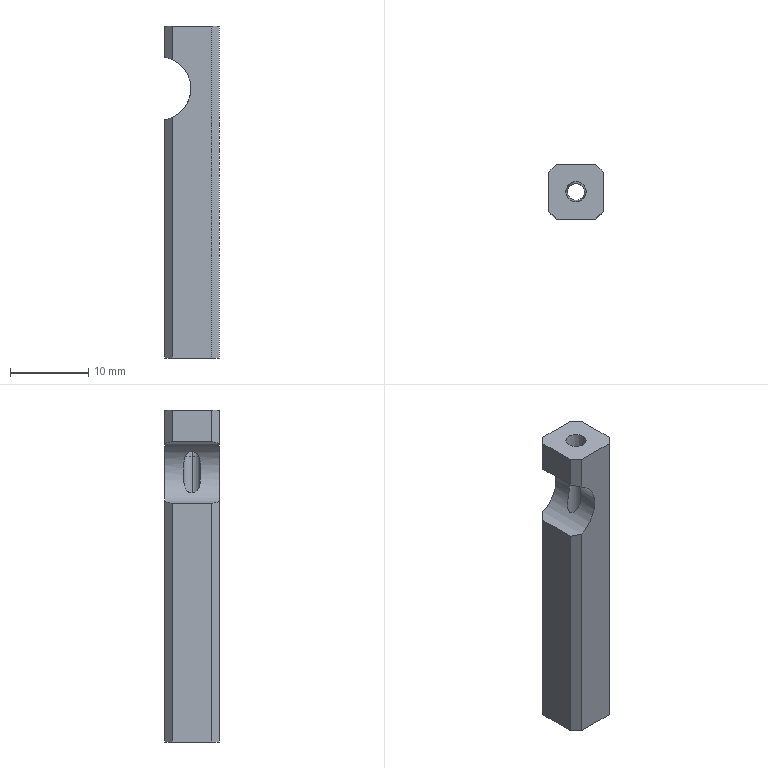Part | SolidWorks | features Chamfer 3, ICE 3, Extrusion 1, MoveFace 1 | 1 solid | 18 faces | box 7 x 7 x 42.5 mm | volume 1702 mm3 | plane 13 | cylinder 3 | cone 2 | commonest cylinder face diameters 2.2 x2 8.159 x1
STEP:
#1=CARTESIAN_POINT('',(-1.122,0.,37.161));
#2=VERTEX_POINT('',#1);
#3=CARTESIAN_POINT('',(-0.6584,-0.8812,36.5));
#4=VERTEX_POINT('',#3);
#5=CARTESIAN_POINT('',(-1.122,0.,37.161));
#6=CARTESIAN_POINT('',(-1.122,-0.1059,37.161));
#7=CARTESIAN_POINT('',(-1.106,-0.2127,37.142));
#8=CARTESIAN_POINT('',(-1.048,-0.4063,37.073));
#9=CARTESIAN_POINT('',(-1.007,-0.4931,37.022));
#10=CARTESIAN_POINT('',(-0.8673,-0.7166,36.838));
#11=CARTESIAN_POINT('',(-0.7581,-0.8141,36.677));
#12=CARTESIAN_POINT('',(-0.6584,-0.8812,36.5));
#13=B_SPLINE_CURVE_WITH_KNOTS('',3,(#5,#6,#7,#8,#9,#10,#11,#12),.UNSPECIFIED.,.F.,.F.,(4,2,2,4),(0.001267,0.001583,0.001898,0.002528),.UNSPECIFIED.);
#14=EDGE_CURVE('',#2,#4,#13,.T.);
#15=ORIENTED_EDGE('',*,*,#14,.F.);
#16=CARTESIAN_POINT('',(-1.3,0.,42.5));
#17=VERTEX_POINT('',#16);
#18=CARTESIAN_POINT('',(-1.1,0.,36.5));
#19=DIRECTION('',(-0.03331,0.,0.9994));
#20=VECTOR('',#19,1000.);
#21=LINE('',#18,#20);
#22=EDGE_CURVE('',#2,#17,#21,.T.);
#23=ORIENTED_EDGE('',*,*,#22,.T.);
#24=CARTESIAN_POINT('',(1.3,0.,42.5));
#25=VERTEX_POINT('',#24);
#26=CARTESIAN_POINT('',(0.,0.,42.5));
#27=DIRECTION('',(0.,0.,-1.));
#28=DIRECTION('',(1.,0.,0.));
#29=AXIS2_PLACEMENT_3D('',#26,#27,#28);
#30=CIRCLE('',#29,1.3);
#31=EDGE_CURVE('',#25,#17,#30,.T.);
#32=ORIENTED_EDGE('',*,*,#31,.F.);
#33=CARTESIAN_POINT('',(1.1,0.,36.5));
#34=VERTEX_POINT('',#33);
#35=CARTESIAN_POINT('',(1.1,0.,36.5));
#36=DIRECTION('',(0.03331,0.,0.9994));
#37=VECTOR('',#36,1000.);
#38=LINE('',#35,#37);
#39=EDGE_CURVE('',#34,#25,#38,.T.);
#40=ORIENTED_EDGE('',*,*,#39,.F.);
#41=CARTESIAN_POINT('',(0.,0.,36.5));
#42=DIRECTION('',(0.,0.,1.));
#43=DIRECTION('',(1.,0.,0.));
#44=AXIS2_PLACEMENT_3D('',#41,#42,#43);
#45=CIRCLE('',#44,1.1);
#46=EDGE_CURVE('',#4,#34,#45,.T.);
#47=ORIENTED_EDGE('',*,*,#46,.F.);
#48=EDGE_LOOP('',(#15,#23,#32,#40,#47));
#49=FACE_OUTER_BOUND('',#48,.T.);
#50=CARTESIAN_POINT('',(0.,0.,36.5));
#51=DIRECTION('',(0.,0.,1.));
#52=DIRECTION('',(1.,0.,0.));
#53=AXIS2_PLACEMENT_3D('',#50,#51,#52);
#54=CONICAL_SURFACE('',#53,1.1,0.03332);
#55=ADVANCED_FACE('',(#49),#54,.F.);
#56=ORIENTED_EDGE('',*,*,#46,.T.);
#57=CARTESIAN_POINT('',(1.1,0.,0.));
#58=VERTEX_POINT('',#57);
#59=CARTESIAN_POINT('',(1.1,0.,40.));
#60=DIRECTION('',(0.,0.,-1.));
#61=VECTOR('',#60,1000.);
#62=LINE('',#59,#61);
#63=EDGE_CURVE('',#34,#58,#62,.T.);
#64=ORIENTED_EDGE('',*,*,#63,.T.);
#65=CARTESIAN_POINT('',(-1.1,0.,0.));
#66=VERTEX_POINT('',#65);
#67=CARTESIAN_POINT('',(0.,0.,0.));
#68=DIRECTION('',(0.,0.,1.));
#69=DIRECTION('',(1.,0.,0.));
#70=AXIS2_PLACEMENT_3D('',#67,#68,#69);
#71=CIRCLE('',#70,1.1);
#72=EDGE_CURVE('',#66,#58,#71,.T.);
#73=ORIENTED_EDGE('',*,*,#72,.F.);
#74=CARTESIAN_POINT('',(-1.1,0.,31.865));
#75=VERTEX_POINT('',#74);
#76=CARTESIAN_POINT('',(-1.1,0.,40.));
#77=DIRECTION('',(0.,0.,-1.));
#78=VECTOR('',#77,1000.);
#79=LINE('',#76,#78);
#80=EDGE_CURVE('',#75,#66,#79,.T.);
#81=ORIENTED_EDGE('',*,*,#80,.F.);
#82=CARTESIAN_POINT('',(-0.6584,-0.8812,36.5));
#83=CARTESIAN_POINT('',(-0.6059,-0.9204,36.407));
#84=CARTESIAN_POINT('',(-0.555,-0.9512,36.307));
#85=CARTESIAN_POINT('',(-0.4617,-0.9998,36.105));
#86=CARTESIAN_POINT('',(-0.419,-1.018,36.001));
#87=CARTESIAN_POINT('',(-0.3034,-1.061,35.683));
#88=CARTESIAN_POINT('',(-0.2428,-1.074,35.461));
#89=CARTESIAN_POINT('',(-0.1607,-1.089,35.014));
#90=CARTESIAN_POINT('',(-0.1385,-1.091,34.789));
#91=CARTESIAN_POINT('',(-0.1316,-1.092,34.336));
#92=CARTESIAN_POINT('',(-0.1473,-1.091,34.106));
#93=CARTESIAN_POINT('',(-0.2161,-1.079,33.657));
#94=CARTESIAN_POINT('',(-0.2688,-1.069,33.438));
#95=CARTESIAN_POINT('',(-0.4097,-1.024,33.01));
#96=CARTESIAN_POINT('',(-0.4996,-0.9875,32.799));
#97=CARTESIAN_POINT('',(-0.6524,-0.8878,32.508));
#98=CARTESIAN_POINT('',(-0.7068,-0.8462,32.414));
#99=CARTESIAN_POINT('',(-0.8149,-0.7426,32.242));
#100=CARTESIAN_POINT('',(-0.869,-0.6808,32.163));
#101=CARTESIAN_POINT('',(-0.9706,-0.5258,32.024));
#102=CARTESIAN_POINT('',(-1.016,-0.435,31.967));
#103=CARTESIAN_POINT('',(-1.065,-0.2806,31.906));
#104=CARTESIAN_POINT('',(-1.078,-0.2271,31.891));
#105=CARTESIAN_POINT('',(-1.095,-0.1158,31.87));
#106=CARTESIAN_POINT('',(-1.1,-0.05736,31.865));
#107=CARTESIAN_POINT('',(-1.1,0.,31.865));
#108=B_SPLINE_CURVE_WITH_KNOTS('',3,(#82,#83,#84,#85,#86,#87,#88,#89,#90,#91,#92,#93,#94,#95,#96,#97,#98,#99,#100,#101,#102,#103,#104,#105,#106,#107),.UNSPECIFIED.,.F.,.F.,(4,2,2,2,2,2,2,2,2,2,2,2,4),(0.001246,0.001589,0.001932,0.002617,0.003303,0.003989,0.004675,0.00536,0.005703,0.006046,0.006389,0.00656,0.006732),.UNSPECIFIED.);
#109=EDGE_CURVE('',#4,#75,#108,.T.);
#110=ORIENTED_EDGE('',*,*,#109,.F.);
#111=EDGE_LOOP('',(#56,#64,#73,#81,#110));
#112=FACE_OUTER_BOUND('',#111,.T.);
#113=CARTESIAN_POINT('',(0.,0.,40.));
#114=DIRECTION('',(0.,0.,-1.));
#115=DIRECTION('',(-1.,0.,0.));
#116=AXIS2_PLACEMENT_3D('',#113,#114,#115);
#117=CYLINDRICAL_SURFACE('',#116,1.1);
#118=ADVANCED_FACE('',(#112),#117,.F.);
#119=CARTESIAN_POINT('',(-3.5,2.5,30.483));
#120=VERTEX_POINT('',#119);
#121=CARTESIAN_POINT('',(-3.5,-2.5,30.483));
#122=VERTEX_POINT('',#121);
#123=CARTESIAN_POINT('',(-3.5,-9.5,30.483));
#124=DIRECTION('',(0.,-1.,0.));
#125=VECTOR('',#124,1000.);
#126=LINE('',#123,#125);
#127=EDGE_CURVE('',#120,#122,#126,.T.);
#128=ORIENTED_EDGE('',*,*,#127,.F.);
#129=CARTESIAN_POINT('',(-3.5,2.5,0.));
#130=VERTEX_POINT('',#129);
#131=CARTESIAN_POINT('',(-3.5,2.5,-9.899));
#132=DIRECTION('',(0.,0.,-1.));
#133=VECTOR('',#132,1000.);
#134=LINE('',#131,#133);
#135=EDGE_CURVE('',#120,#130,#134,.T.);
#136=ORIENTED_EDGE('',*,*,#135,.T.);
#137=CARTESIAN_POINT('',(-3.5,-2.5,0.));
#138=VERTEX_POINT('',#137);
#139=CARTESIAN_POINT('',(-3.5,-3.5,0.));
#140=DIRECTION('',(0.,1.,0.));
#141=VECTOR('',#140,1000.);
#142=LINE('',#139,#141);
#143=EDGE_CURVE('',#138,#130,#142,.T.);
#144=ORIENTED_EDGE('',*,*,#143,.F.);
#145=CARTESIAN_POINT('',(-3.5,-2.5,-9.899));
#146=DIRECTION('',(0.,0.,1.));
#147=VECTOR('',#146,1000.);
#148=LINE('',#145,#147);
#149=EDGE_CURVE('',#138,#122,#148,.T.);
#150=ORIENTED_EDGE('',*,*,#149,.T.);
#151=EDGE_LOOP('',(#128,#136,#144,#150));
#152=FACE_OUTER_BOUND('',#151,.T.);
#153=CARTESIAN_POINT('',(-3.5,-3.5,-9.899));
#154=DIRECTION('',(-1.,0.,0.));
#155=DIRECTION('',(0.,0.,1.));
#156=AXIS2_PLACEMENT_3D('',#153,#154,#155);
#157=PLANE('',#156);
#158=ADVANCED_FACE('',(#152),#157,.T.);
#159=CARTESIAN_POINT('',(-2.5,3.5,30.798));
#160=VERTEX_POINT('',#159);
#161=CARTESIAN_POINT('',(-2.5,3.5,30.798));
#162=CARTESIAN_POINT('',(-2.819,3.181,30.65));
#163=CARTESIAN_POINT('',(-3.154,2.846,30.545));
#164=CARTESIAN_POINT('',(-3.5,2.5,30.483));
#165=(BOUNDED_CURVE()B_SPLINE_CURVE(3,(#161,#162,#163,#164),.UNSPECIFIED.,.F.,.T.)B_SPLINE_CURVE_WITH_KNOTS((4,4),(1.137,1.395),.UNSPECIFIED.)CURVE()GEOMETRIC_REPRESENTATION_ITEM()RATIONAL_B_SPLINE_CURVE((1.,0.9945,0.9945,1.))REPRESENTATION_ITEM(''));
#166=EDGE_CURVE('',#160,#120,#165,.T.);
#167=ORIENTED_EDGE('',*,*,#166,.F.);
#168=CARTESIAN_POINT('',(-2.5,3.5,0.));
#169=VERTEX_POINT('',#168);
#170=CARTESIAN_POINT('',(-2.5,3.5,-9.899));
#171=DIRECTION('',(0.,0.,1.));
#172=VECTOR('',#171,1000.);
#173=LINE('',#170,#172);
#174=EDGE_CURVE('',#169,#160,#173,.T.);
#175=ORIENTED_EDGE('',*,*,#174,.F.);
#176=CARTESIAN_POINT('',(-2.5,3.5,0.));
#177=DIRECTION('',(0.7071,0.7071,0.));
#178=VECTOR('',#177,1000.);
#179=LINE('',#176,#178);
#180=EDGE_CURVE('',#130,#169,#179,.T.);
#181=ORIENTED_EDGE('',*,*,#180,.F.);
#182=ORIENTED_EDGE('',*,*,#135,.F.);
#183=EDGE_LOOP('',(#167,#175,#181,#182));
#184=FACE_OUTER_BOUND('',#183,.T.);
#185=CARTESIAN_POINT('',(-2.5,3.5,-9.899));
#186=DIRECTION('',(0.7071,-0.7071,0.));
#187=DIRECTION('',(0.,0.,1.));
#188=AXIS2_PLACEMENT_3D('',#185,#186,#187);
#189=PLANE('',#188);
#190=ADVANCED_FACE('',(#184),#189,.F.);
#191=CARTESIAN_POINT('',(-2.5,-3.5,30.798));
#192=VERTEX_POINT('',#191);
#193=CARTESIAN_POINT('',(-3.5,-2.5,30.483));
#194=CARTESIAN_POINT('',(-3.154,-2.846,30.545));
#195=CARTESIAN_POINT('',(-2.819,-3.181,30.65));
#196=CARTESIAN_POINT('',(-2.5,-3.5,30.798));
#197=(BOUNDED_CURVE()B_SPLINE_CURVE(3,(#193,#194,#195,#196),.UNSPECIFIED.,.F.,.T.)B_SPLINE_CURVE_WITH_KNOTS((4,4),(1.747,2.004),.UNSPECIFIED.)CURVE()GEOMETRIC_REPRESENTATION_ITEM()RATIONAL_B_SPLINE_CURVE((1.,0.9945,0.9945,1.))REPRESENTATION_ITEM(''));
#198=EDGE_CURVE('',#122,#192,#197,.T.);
#199=ORIENTED_EDGE('',*,*,#198,.F.);
#200=ORIENTED_EDGE('',*,*,#149,.F.);
#201=CARTESIAN_POINT('',(-2.5,-3.5,0.));
#202=VERTEX_POINT('',#201);
#203=CARTESIAN_POINT('',(-3.5,-2.5,0.));
#204=DIRECTION('',(-0.7071,0.7071,0.));
#205=VECTOR('',#204,1000.);
#206=LINE('',#203,#205);
#207=EDGE_CURVE('',#202,#138,#206,.T.);
#208=ORIENTED_EDGE('',*,*,#207,.F.);
#209=CARTESIAN_POINT('',(-2.5,-3.5,-9.899));
#210=DIRECTION('',(0.,0.,-1.));
#211=VECTOR('',#210,1000.);
#212=LINE('',#209,#211);
#213=EDGE_CURVE('',#192,#202,#212,.T.);
#214=ORIENTED_EDGE('',*,*,#213,.F.);
#215=EDGE_LOOP('',(#199,#200,#208,#214));
#216=FACE_OUTER_BOUND('',#215,.T.);
#217=CARTESIAN_POINT('',(-3.5,-2.5,-9.899));
#218=DIRECTION('',(0.7071,0.7071,0.));
#219=DIRECTION('',(0.,0.,1.));
#220=AXIS2_PLACEMENT_3D('',#217,#218,#219);
#221=PLANE('',#220);
#222=ADVANCED_FACE('',(#216),#221,.F.);
#223=ORIENTED_EDGE('',*,*,#31,.T.);
#224=CARTESIAN_POINT('',(0.,0.,42.5));
#225=DIRECTION('',(0.,0.,-1.));
#226=DIRECTION('',(1.,0.,0.));
#227=AXIS2_PLACEMENT_3D('',#224,#225,#226);
#228=CIRCLE('',#227,1.3);
#229=EDGE_CURVE('',#17,#25,#228,.T.);
#230=ORIENTED_EDGE('',*,*,#229,.T.);
#231=EDGE_LOOP('',(#223,#230));
#232=FACE_BOUND('',#231,.T.);
#233=CARTESIAN_POINT('',(3.5,-2.5,42.5));
#234=VERTEX_POINT('',#233);
#235=CARTESIAN_POINT('',(3.5,2.5,42.5));
#236=VERTEX_POINT('',#235);
#237=CARTESIAN_POINT('',(3.5,0.,42.5));
#238=DIRECTION('',(0.,1.,0.));
#239=VECTOR('',#238,1000.);
#240=LINE('',#237,#239);
#241=EDGE_CURVE('',#234,#236,#240,.T.);
#242=ORIENTED_EDGE('',*,*,#241,.T.);
#243=CARTESIAN_POINT('',(2.5,3.5,42.5));
#244=VERTEX_POINT('',#243);
#245=CARTESIAN_POINT('',(3.,3.,42.5));
#246=DIRECTION('',(-0.7071,0.7071,0.));
#247=VECTOR('',#246,1000.);
#248=LINE('',#245,#247);
#249=EDGE_CURVE('',#236,#244,#248,.T.);
#250=ORIENTED_EDGE('',*,*,#249,.T.);
#251=CARTESIAN_POINT('',(-2.5,3.5,42.5));
#252=VERTEX_POINT('',#251);
#253=CARTESIAN_POINT('',(0.,3.5,42.5));
#254=DIRECTION('',(-1.,0.,0.));
#255=VECTOR('',#254,1000.);
#256=LINE('',#253,#255);
#257=EDGE_CURVE('',#244,#252,#256,.T.);
#258=ORIENTED_EDGE('',*,*,#257,.T.);
#259=CARTESIAN_POINT('',(-3.5,2.5,42.5));
#260=VERTEX_POINT('',#259);
#261=CARTESIAN_POINT('',(-3.,3.,42.5));
#262=DIRECTION('',(-0.7071,-0.7071,0.));
#263=VECTOR('',#262,1000.);
#264=LINE('',#261,#263);
#265=EDGE_CURVE('',#252,#260,#264,.T.);
#266=ORIENTED_EDGE('',*,*,#265,.T.);
#267=CARTESIAN_POINT('',(-3.5,-2.5,42.5));
#268=VERTEX_POINT('',#267);
#269=CARTESIAN_POINT('',(-3.5,0.,42.5));
#270=DIRECTION('',(0.,-1.,0.));
#271=VECTOR('',#270,1000.);
#272=LINE('',#269,#271);
#273=EDGE_CURVE('',#260,#268,#272,.T.);
#274=ORIENTED_EDGE('',*,*,#273,.T.);
#275=CARTESIAN_POINT('',(-2.5,-3.5,42.5));
#276=VERTEX_POINT('',#275);
#277=CARTESIAN_POINT('',(-3.,-3.,42.5));
#278=DIRECTION('',(0.7071,-0.7071,0.));
#279=VECTOR('',#278,1000.);
#280=LINE('',#277,#279);
#281=EDGE_CURVE('',#268,#276,#280,.T.);
#282=ORIENTED_EDGE('',*,*,#281,.T.);
#283=CARTESIAN_POINT('',(2.5,-3.5,42.5));
#284=VERTEX_POINT('',#283);
#285=CARTESIAN_POINT('',(0.,-3.5,42.5));
#286=DIRECTION('',(1.,0.,0.));
#287=VECTOR('',#286,1000.);
#288=LINE('',#285,#287);
#289=EDGE_CURVE('',#276,#284,#288,.T.);
#290=ORIENTED_EDGE('',*,*,#289,.T.);
#291=CARTESIAN_POINT('',(3.,-3.,42.5));
#292=DIRECTION('',(0.7071,0.7071,0.));
#293=VECTOR('',#292,1000.);
#294=LINE('',#291,#293);
#295=EDGE_CURVE('',#284,#234,#294,.T.);
#296=ORIENTED_EDGE('',*,*,#295,.T.);
#297=EDGE_LOOP('',(#242,#250,#258,#266,#274,#282,#290,#296));
#298=FACE_OUTER_BOUND('',#297,.T.);
#299=CARTESIAN_POINT('',(0.,0.,42.5));
#300=DIRECTION('',(0.,0.,1.));
#301=DIRECTION('',(1.,0.,0.));
#302=AXIS2_PLACEMENT_3D('',#299,#300,#301);
#303=PLANE('',#302);
#304=ADVANCED_FACE('',(#232,#298),#303,.T.);
#305=CARTESIAN_POINT('',(2.5,3.5,0.));
#306=VERTEX_POINT('',#305);
#307=CARTESIAN_POINT('',(-3.5,3.5,0.));
#308=DIRECTION('',(1.,0.,0.));
#309=VECTOR('',#308,1000.);
#310=LINE('',#307,#309);
#311=EDGE_CURVE('',#169,#306,#310,.T.);
#312=ORIENTED_EDGE('',*,*,#311,.T.);
#313=CARTESIAN_POINT('',(3.5,2.5,0.));
#314=VERTEX_POINT('',#313);
#315=CARTESIAN_POINT('',(3.5,2.5,0.));
#316=DIRECTION('',(0.7071,-0.7071,0.));
#317=VECTOR('',#316,1000.);
#318=LINE('',#315,#317);
#319=EDGE_CURVE('',#306,#314,#318,.T.);
#320=ORIENTED_EDGE('',*,*,#319,.T.);
#321=CARTESIAN_POINT('',(3.5,-2.5,0.));
#322=VERTEX_POINT('',#321);
#323=CARTESIAN_POINT('',(3.5,-3.5,0.));
#324=DIRECTION('',(0.,-1.,0.));
#325=VECTOR('',#324,1000.);
#326=LINE('',#323,#325);
#327=EDGE_CURVE('',#314,#322,#326,.T.);
#328=ORIENTED_EDGE('',*,*,#327,.T.);
#329=CARTESIAN_POINT('',(2.5,-3.5,0.));
#330=VERTEX_POINT('',#329);
#331=CARTESIAN_POINT('',(2.5,-3.5,0.));
#332=DIRECTION('',(-0.7071,-0.7071,0.));
#333=VECTOR('',#332,1000.);
#334=LINE('',#331,#333);
#335=EDGE_CURVE('',#322,#330,#334,.T.);
#336=ORIENTED_EDGE('',*,*,#335,.T.);
#337=CARTESIAN_POINT('',(-3.5,-3.5,0.));
#338=DIRECTION('',(-1.,0.,0.));
#339=VECTOR('',#338,1000.);
#340=LINE('',#337,#339);
#341=EDGE_CURVE('',#330,#202,#340,.T.);
#342=ORIENTED_EDGE('',*,*,#341,.T.);
#343=ORIENTED_EDGE('',*,*,#207,.T.);
#344=ORIENTED_EDGE('',*,*,#143,.T.);
#345=ORIENTED_EDGE('',*,*,#180,.T.);
#346=EDGE_LOOP('',(#312,#320,#328,#336,#342,#343,#344,#345));
#347=FACE_OUTER_BOUND('',#346,.T.);
#348=ORIENTED_EDGE('',*,*,#72,.T.);
#349=CARTESIAN_POINT('',(0.,0.,0.));
#350=DIRECTION('',(0.,0.,1.));
#351=DIRECTION('',(1.,0.,0.));
#352=AXIS2_PLACEMENT_3D('',#349,#350,#351);
#353=CIRCLE('',#352,1.1);
#354=EDGE_CURVE('',#58,#66,#353,.T.);
#355=ORIENTED_EDGE('',*,*,#354,.T.);
#356=EDGE_LOOP('',(#348,#355));
#357=FACE_BOUND('',#356,.T.);
#358=CARTESIAN_POINT('',(0.,0.,0.));
#359=DIRECTION('',(0.,0.,1.));
#360=DIRECTION('',(1.,0.,0.));
#361=AXIS2_PLACEMENT_3D('',#358,#359,#360);
#362=PLANE('',#361);
#363=ADVANCED_FACE('',(#347,#357),#362,.F.);
#364=ORIENTED_EDGE('',*,*,#63,.F.);
#365=CARTESIAN_POINT('',(-0.6584,0.8812,36.5));
#366=VERTEX_POINT('',#365);
#367=CARTESIAN_POINT('',(0.,0.,36.5));
#368=DIRECTION('',(0.,0.,1.));
#369=DIRECTION('',(1.,0.,0.));
#370=AXIS2_PLACEMENT_3D('',#367,#368,#369);
#371=CIRCLE('',#370,1.1);
#372=EDGE_CURVE('',#34,#366,#371,.T.);
#373=ORIENTED_EDGE('',*,*,#372,.T.);
#374=CARTESIAN_POINT('',(-1.1,0.,31.865));
#375=CARTESIAN_POINT('',(-1.1,0.1143,31.865));
#376=CARTESIAN_POINT('',(-1.081,0.2291,31.886));
#377=CARTESIAN_POINT('',(-1.016,0.4346,31.966));
#378=CARTESIAN_POINT('',(-0.9706,0.5258,32.024));
#379=CARTESIAN_POINT('',(-0.8188,0.7573,32.232));
#380=CARTESIAN_POINT('',(-0.703,0.8546,32.411));
#381=CARTESIAN_POINT('',(-0.5007,0.9868,32.797));
#382=CARTESIAN_POINT('',(-0.4107,1.023,33.007));
#383=CARTESIAN_POINT('',(-0.2692,1.069,33.436));
#384=CARTESIAN_POINT('',(-0.2163,1.079,33.656));
#385=CARTESIAN_POINT('',(-0.1472,1.091,34.107));
#386=CARTESIAN_POINT('',(-0.1316,1.092,34.335));
#387=CARTESIAN_POINT('',(-0.1385,1.091,34.788));
#388=CARTESIAN_POINT('',(-0.1607,1.089,35.015));
#389=CARTESIAN_POINT('',(-0.2436,1.074,35.464));
#390=CARTESIAN_POINT('',(-0.3033,1.061,35.683));
#391=CARTESIAN_POINT('',(-0.4574,1.004,36.106));
#392=CARTESIAN_POINT('',(-0.5533,0.9598,36.313));
#393=CARTESIAN_POINT('',(-0.6584,0.8812,36.5));
#394=B_SPLINE_CURVE_WITH_KNOTS('',3,(#374,#375,#376,#377,#378,#379,#380,#381,#382,#383,#384,#385,#386,#387,#388,#389,#390,#391,#392,#393),.UNSPECIFIED.,.F.,.F.,(4,2,2,2,2,2,2,2,2,4),(0.006732,0.007073,0.007415,0.008098,0.008782,0.009465,0.01015,0.01083,0.01152,0.0122),.UNSPECIFIED.);
#395=EDGE_CURVE('',#75,#366,#394,.T.);
#396=ORIENTED_EDGE('',*,*,#395,.F.);
#397=ORIENTED_EDGE('',*,*,#80,.T.);
#398=ORIENTED_EDGE('',*,*,#354,.F.);
#399=EDGE_LOOP('',(#364,#373,#396,#397,#398));
#400=FACE_OUTER_BOUND('',#399,.T.);
#401=CARTESIAN_POINT('',(0.,0.,40.));
#402=DIRECTION('',(0.,0.,-1.));
#403=DIRECTION('',(-1.,0.,0.));
#404=AXIS2_PLACEMENT_3D('',#401,#402,#403);
#405=CYLINDRICAL_SURFACE('',#404,1.1);
#406=ADVANCED_FACE('',(#400),#405,.F.);
#407=CARTESIAN_POINT('',(-2.5,3.5,38.202));
#408=VERTEX_POINT('',#407);
#409=CARTESIAN_POINT('',(-4.214,3.5,34.5));
#410=DIRECTION('',(0.,1.,0.));
#411=DIRECTION('',(0.,0.,1.));
#412=AXIS2_PLACEMENT_3D('',#409,#410,#411);
#413=CIRCLE('',#412,4.08);
#414=EDGE_CURVE('',#408,#160,#413,.T.);
#415=ORIENTED_EDGE('',*,*,#414,.F.);
#416=CARTESIAN_POINT('',(-2.5,3.5,-9.899));
#417=DIRECTION('',(0.,0.,1.));
#418=VECTOR('',#417,1000.);
#419=LINE('',#416,#418);
#420=EDGE_CURVE('',#408,#252,#419,.T.);
#421=ORIENTED_EDGE('',*,*,#420,.T.);
#422=ORIENTED_EDGE('',*,*,#257,.F.);
#423=CARTESIAN_POINT('',(2.5,3.5,-9.899));
#424=DIRECTION('',(0.,0.,-1.));
#425=VECTOR('',#424,1000.);
#426=LINE('',#423,#425);
#427=EDGE_CURVE('',#244,#306,#426,.T.);
#428=ORIENTED_EDGE('',*,*,#427,.T.);
#429=ORIENTED_EDGE('',*,*,#311,.F.);
#430=ORIENTED_EDGE('',*,*,#174,.T.);
#431=EDGE_LOOP('',(#415,#421,#422,#428,#429,#430));
#432=FACE_OUTER_BOUND('',#431,.T.);
#433=CARTESIAN_POINT('',(-3.5,3.5,-9.899));
#434=DIRECTION('',(0.,1.,0.));
#435=DIRECTION('',(0.,0.,1.));
#436=AXIS2_PLACEMENT_3D('',#433,#434,#435);
#437=PLANE('',#436);
#438=ADVANCED_FACE('',(#432),#437,.T.);
#439=CARTESIAN_POINT('',(-3.5,-2.5,38.517));
#440=VERTEX_POINT('',#439);
#441=CARTESIAN_POINT('',(-3.5,2.5,38.517));
#442=VERTEX_POINT('',#441);
#443=CARTESIAN_POINT('',(-3.5,-9.5,38.517));
#444=DIRECTION('',(0.,1.,0.));
#445=VECTOR('',#444,1000.);
#446=LINE('',#443,#445);
#447=EDGE_CURVE('',#440,#442,#446,.T.);
#448=ORIENTED_EDGE('',*,*,#447,.F.);
#449=CARTESIAN_POINT('',(-3.5,-2.5,-9.899));
#450=DIRECTION('',(0.,0.,1.));
#451=VECTOR('',#450,1000.);
#452=LINE('',#449,#451);
#453=EDGE_CURVE('',#440,#268,#452,.T.);
#454=ORIENTED_EDGE('',*,*,#453,.T.);
#455=ORIENTED_EDGE('',*,*,#273,.F.);
#456=CARTESIAN_POINT('',(-3.5,2.5,-9.899));
#457=DIRECTION('',(0.,0.,-1.));
#458=VECTOR('',#457,1000.);
#459=LINE('',#456,#458);
#460=EDGE_CURVE('',#260,#442,#459,.T.);
#461=ORIENTED_EDGE('',*,*,#460,.T.);
#462=EDGE_LOOP('',(#448,#454,#455,#461));
#463=FACE_OUTER_BOUND('',#462,.T.);
#464=CARTESIAN_POINT('',(-3.5,-3.5,-9.899));
#465=DIRECTION('',(-1.,0.,0.));
#466=DIRECTION('',(0.,0.,1.));
#467=AXIS2_PLACEMENT_3D('',#464,#465,#466);
#468=PLANE('',#467);
#469=ADVANCED_FACE('',(#463),#468,.T.);
#470=CARTESIAN_POINT('',(-2.5,-3.5,38.202));
#471=VERTEX_POINT('',#470);
#472=CARTESIAN_POINT('',(-4.214,-3.5,34.5));
#473=DIRECTION('',(0.,-1.,0.));
#474=DIRECTION('',(0.,0.,-1.));
#475=AXIS2_PLACEMENT_3D('',#472,#473,#474);
#476=CIRCLE('',#475,4.08);
#477=EDGE_CURVE('',#192,#471,#476,.T.);
#478=ORIENTED_EDGE('',*,*,#477,.F.);
#479=ORIENTED_EDGE('',*,*,#213,.T.);
#480=ORIENTED_EDGE('',*,*,#341,.F.);
#481=CARTESIAN_POINT('',(2.5,-3.5,-9.899));
#482=DIRECTION('',(0.,0.,1.));
#483=VECTOR('',#482,1000.);
#484=LINE('',#481,#483);
#485=EDGE_CURVE('',#330,#284,#484,.T.);
#486=ORIENTED_EDGE('',*,*,#485,.T.);
#487=ORIENTED_EDGE('',*,*,#289,.F.);
#488=CARTESIAN_POINT('',(-2.5,-3.5,-9.899));
#489=DIRECTION('',(0.,0.,-1.));
#490=VECTOR('',#489,1000.);
#491=LINE('',#488,#490);
#492=EDGE_CURVE('',#276,#471,#491,.T.);
#493=ORIENTED_EDGE('',*,*,#492,.T.);
#494=EDGE_LOOP('',(#478,#479,#480,#486,#487,#493));
#495=FACE_OUTER_BOUND('',#494,.T.);
#496=CARTESIAN_POINT('',(-3.5,-3.5,-9.899));
#497=DIRECTION('',(0.,-1.,0.));
#498=DIRECTION('',(0.,0.,-1.));
#499=AXIS2_PLACEMENT_3D('',#496,#497,#498);
#500=PLANE('',#499);
#501=ADVANCED_FACE('',(#495),#500,.T.);
#502=ORIENTED_EDGE('',*,*,#327,.F.);
#503=CARTESIAN_POINT('',(3.5,2.5,-9.899));
#504=DIRECTION('',(0.,0.,1.));
#505=VECTOR('',#504,1000.);
#506=LINE('',#503,#505);
#507=EDGE_CURVE('',#314,#236,#506,.T.);
#508=ORIENTED_EDGE('',*,*,#507,.T.);
#509=ORIENTED_EDGE('',*,*,#241,.F.);
#510=CARTESIAN_POINT('',(3.5,-2.5,-9.899));
#511=DIRECTION('',(0.,0.,-1.));
#512=VECTOR('',#511,1000.);
#513=LINE('',#510,#512);
#514=EDGE_CURVE('',#234,#322,#513,.T.);
#515=ORIENTED_EDGE('',*,*,#514,.T.);
#516=EDGE_LOOP('',(#502,#508,#509,#515));
#517=FACE_OUTER_BOUND('',#516,.T.);
#518=CARTESIAN_POINT('',(3.5,-3.5,-9.899));
#519=DIRECTION('',(1.,0.,0.));
#520=DIRECTION('',(0.,0.,-1.));
#521=AXIS2_PLACEMENT_3D('',#518,#519,#520);
#522=PLANE('',#521);
#523=ADVANCED_FACE('',(#517),#522,.T.);
#524=ORIENTED_EDGE('',*,*,#319,.F.);
#525=ORIENTED_EDGE('',*,*,#427,.F.);
#526=ORIENTED_EDGE('',*,*,#249,.F.);
#527=ORIENTED_EDGE('',*,*,#507,.F.);
#528=EDGE_LOOP('',(#524,#525,#526,#527));
#529=FACE_OUTER_BOUND('',#528,.T.);
#530=CARTESIAN_POINT('',(3.5,2.5,-9.899));
#531=DIRECTION('',(-0.7071,-0.7071,0.));
#532=DIRECTION('',(0.,0.,1.));
#533=AXIS2_PLACEMENT_3D('',#530,#531,#532);
#534=PLANE('',#533);
#535=ADVANCED_FACE('',(#529),#534,.F.);
#536=CARTESIAN_POINT('',(-3.5,2.5,38.517));
#537=CARTESIAN_POINT('',(-3.154,2.846,38.455));
#538=CARTESIAN_POINT('',(-2.819,3.181,38.35));
#539=CARTESIAN_POINT('',(-2.5,3.5,38.202));
#540=(BOUNDED_CURVE()B_SPLINE_CURVE(3,(#536,#537,#538,#539),.UNSPECIFIED.,.F.,.T.)B_SPLINE_CURVE_WITH_KNOTS((4,4),(4.888,5.146),.UNSPECIFIED.)CURVE()GEOMETRIC_REPRESENTATION_ITEM()RATIONAL_B_SPLINE_CURVE((1.,0.9945,0.9945,1.))REPRESENTATION_ITEM(''));
#541=EDGE_CURVE('',#442,#408,#540,.T.);
#542=ORIENTED_EDGE('',*,*,#541,.F.);
#543=ORIENTED_EDGE('',*,*,#460,.F.);
#544=ORIENTED_EDGE('',*,*,#265,.F.);
#545=ORIENTED_EDGE('',*,*,#420,.F.);
#546=EDGE_LOOP('',(#542,#543,#544,#545));
#547=FACE_OUTER_BOUND('',#546,.T.);
#548=CARTESIAN_POINT('',(-2.5,3.5,-9.899));
#549=DIRECTION('',(0.7071,-0.7071,0.));
#550=DIRECTION('',(0.,0.,1.));
#551=AXIS2_PLACEMENT_3D('',#548,#549,#550);
#552=PLANE('',#551);
#553=ADVANCED_FACE('',(#547),#552,.F.);
#554=ORIENTED_EDGE('',*,*,#335,.F.);
#555=ORIENTED_EDGE('',*,*,#514,.F.);
#556=ORIENTED_EDGE('',*,*,#295,.F.);
#557=ORIENTED_EDGE('',*,*,#485,.F.);
#558=EDGE_LOOP('',(#554,#555,#556,#557));
#559=FACE_OUTER_BOUND('',#558,.T.);
#560=CARTESIAN_POINT('',(2.5,-3.5,-9.899));
#561=DIRECTION('',(-0.7071,0.7071,0.));
#562=DIRECTION('',(0.,0.,1.));
#563=AXIS2_PLACEMENT_3D('',#560,#561,#562);
#564=PLANE('',#563);
#565=ADVANCED_FACE('',(#559),#564,.F.);
#566=CARTESIAN_POINT('',(-2.5,-3.5,38.202));
#567=CARTESIAN_POINT('',(-2.819,-3.181,38.35));
#568=CARTESIAN_POINT('',(-3.154,-2.846,38.455));
#569=CARTESIAN_POINT('',(-3.5,-2.5,38.517));
#570=(BOUNDED_CURVE()B_SPLINE_CURVE(3,(#566,#567,#568,#569),.UNSPECIFIED.,.F.,.T.)B_SPLINE_CURVE_WITH_KNOTS((4,4),(4.279,4.536),.UNSPECIFIED.)CURVE()GEOMETRIC_REPRESENTATION_ITEM()RATIONAL_B_SPLINE_CURVE((1.,0.9945,0.9945,1.))REPRESENTATION_ITEM(''));
#571=EDGE_CURVE('',#471,#440,#570,.T.);
#572=ORIENTED_EDGE('',*,*,#571,.F.);
#573=ORIENTED_EDGE('',*,*,#492,.F.);
#574=ORIENTED_EDGE('',*,*,#281,.F.);
#575=ORIENTED_EDGE('',*,*,#453,.F.);
#576=EDGE_LOOP('',(#572,#573,#574,#575));
#577=FACE_OUTER_BOUND('',#576,.T.);
#578=CARTESIAN_POINT('',(-3.5,-2.5,-9.899));
#579=DIRECTION('',(0.7071,0.7071,0.));
#580=DIRECTION('',(0.,0.,1.));
#581=AXIS2_PLACEMENT_3D('',#578,#579,#580);
#582=PLANE('',#581);
#583=ADVANCED_FACE('',(#577),#582,.F.);
#584=ORIENTED_EDGE('',*,*,#477,.T.);
#585=ORIENTED_EDGE('',*,*,#571,.T.);
#586=ORIENTED_EDGE('',*,*,#447,.T.);
#587=ORIENTED_EDGE('',*,*,#541,.T.);
#588=ORIENTED_EDGE('',*,*,#414,.T.);
#589=ORIENTED_EDGE('',*,*,#166,.T.);
#590=ORIENTED_EDGE('',*,*,#127,.T.);
#591=ORIENTED_EDGE('',*,*,#198,.T.);
#592=EDGE_LOOP('',(#584,#585,#586,#587,#588,#589,#590,#591));
#593=FACE_OUTER_BOUND('',#592,.T.);
#594=ORIENTED_EDGE('',*,*,#109,.T.);
#595=ORIENTED_EDGE('',*,*,#395,.T.);
#596=CARTESIAN_POINT('',(-0.6584,0.8812,36.5));
#597=CARTESIAN_POINT('',(-0.7083,0.8476,36.589));
#598=CARTESIAN_POINT('',(-0.7596,0.8068,36.672));
#599=CARTESIAN_POINT('',(-0.8617,0.7048,36.826));
#600=CARTESIAN_POINT('',(-0.9134,0.6425,36.899));
#601=CARTESIAN_POINT('',(-1.006,0.494,37.021));
#602=CARTESIAN_POINT('',(-1.048,0.4063,37.073));
#603=CARTESIAN_POINT('',(-1.105,0.214,37.142));
#604=CARTESIAN_POINT('',(-1.122,0.1065,37.161));
#605=CARTESIAN_POINT('',(-1.122,0.,37.161));
#606=B_SPLINE_CURVE_WITH_KNOTS('',3,(#596,#597,#598,#599,#600,#601,#602,#603,#604,#605),.UNSPECIFIED.,.F.,.F.,(4,2,2,2,4),(0.,0.0003169,0.0006337,0.0009506,0.001267),.UNSPECIFIED.);
#607=EDGE_CURVE('',#366,#2,#606,.T.);
#608=ORIENTED_EDGE('',*,*,#607,.T.);
#609=ORIENTED_EDGE('',*,*,#14,.T.);
#610=EDGE_LOOP('',(#594,#595,#608,#609));
#611=FACE_BOUND('',#610,.T.);
#612=CARTESIAN_POINT('',(-4.214,-9.5,34.5));
#613=DIRECTION('',(0.,1.,0.));
#614=DIRECTION('',(0.,0.,1.));
#615=AXIS2_PLACEMENT_3D('',#612,#613,#614);
#616=CYLINDRICAL_SURFACE('',#615,4.08);
#617=ADVANCED_FACE('',(#593,#611),#616,.F.);
#618=ORIENTED_EDGE('',*,*,#22,.F.);
#619=ORIENTED_EDGE('',*,*,#607,.F.);
#620=ORIENTED_EDGE('',*,*,#372,.F.);
#621=ORIENTED_EDGE('',*,*,#39,.T.);
#622=ORIENTED_EDGE('',*,*,#229,.F.);
#623=EDGE_LOOP('',(#618,#619,#620,#621,#622));
#624=FACE_OUTER_BOUND('',#623,.T.);
#625=CARTESIAN_POINT('',(0.,0.,36.5));
#626=DIRECTION('',(0.,0.,1.));
#627=DIRECTION('',(1.,0.,0.));
#628=AXIS2_PLACEMENT_3D('',#625,#626,#627);
#629=CONICAL_SURFACE('',#628,1.1,0.03332);
#630=ADVANCED_FACE('',(#624),#629,.F.);
#631=CLOSED_SHELL('',(#55,#118,#158,#190,#222,#304,#363,#406,#438,#469,#501,#523,#535,#553,#565,#583,#617,#630));
#632=MANIFOLD_SOLID_BREP('',#631);
#633=CARTESIAN_POINT('',(0.,0.,0.));
#634=DIRECTION('',(0.,0.,1.));
#635=DIRECTION('',(1.,0.,0.));
#636=AXIS2_PLACEMENT_3D('',#633,#634,#635);
#637=(LENGTH_UNIT()NAMED_UNIT(*)SI_UNIT(.MILLI.,.METRE.));
#638=UNCERTAINTY_MEASURE_WITH_UNIT(LENGTH_MEASURE(0.00001),#637,'','');
#639=(NAMED_UNIT(*)PLANE_ANGLE_UNIT()SI_UNIT($,.RADIAN.));
#640=(NAMED_UNIT(*)SI_UNIT($,.STERADIAN.)SOLID_ANGLE_UNIT());
#641=(GEOMETRIC_REPRESENTATION_CONTEXT(3)GLOBAL_UNCERTAINTY_ASSIGNED_CONTEXT((#638))GLOBAL_UNIT_ASSIGNED_CONTEXT((#637,#639,#640))REPRESENTATION_CONTEXT('',''));
#642=ADVANCED_BREP_SHAPE_REPRESENTATION('',(#632,#636),#641);